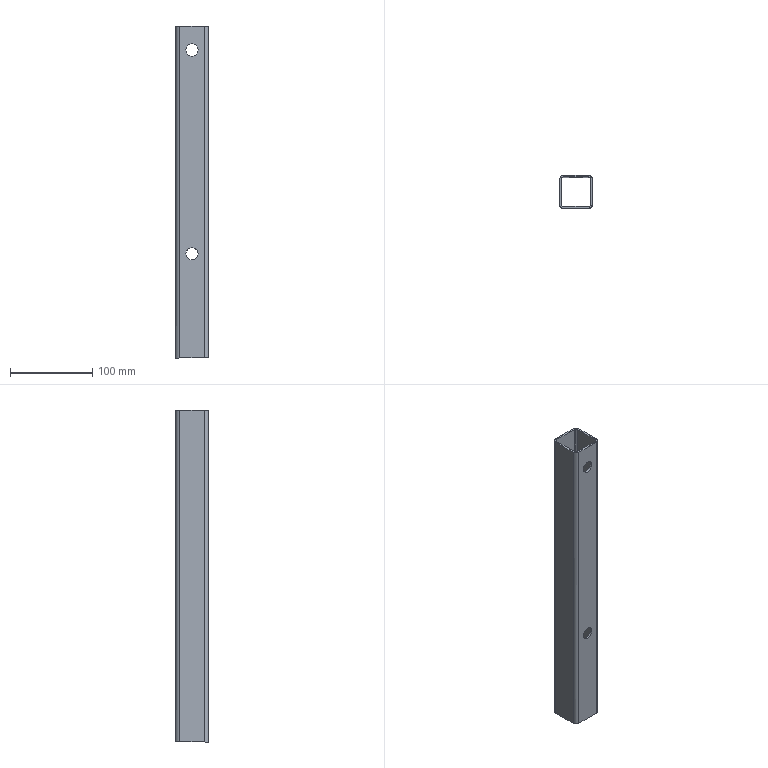Part | NX | features BREP 1 | 1 solid | 30 faces | box 40 x 40 x 404.579 mm | volume 116022 mm3 | cylinder 20 | plane 10 | commonest cylinder face diameters 6 x8 15 x8 10 x4
STEP:
#1=CARTESIAN_POINT('',(2077.08,-390.,484.409));
#2=VERTEX_POINT('',#1);
#3=CARTESIAN_POINT('',(2077.08,-392.,484.409));
#4=VERTEX_POINT('',#3);
#5=CARTESIAN_POINT('',(2077.08,-407.5,484.409));
#6=DIRECTION('',(0.,-1.,0.));
#7=VECTOR('',#6,1000.);
#8=LINE('',#5,#7);
#9=EDGE_CURVE('',#2,#4,#8,.T.);
#10=ORIENTED_EDGE('',*,*,#9,.F.);
#11=CARTESIAN_POINT('',(2092.08,-390.,484.409));
#12=VERTEX_POINT('',#11);
#13=CARTESIAN_POINT('',(2084.58,-390.,484.409));
#14=DIRECTION('',(0.,-1.,0.));
#15=DIRECTION('',(1.,0.,0.));
#16=AXIS2_PLACEMENT_3D('',#13,#14,#15);
#17=CIRCLE('',#16,7.5);
#18=EDGE_CURVE('',#12,#2,#17,.T.);
#19=ORIENTED_EDGE('',*,*,#18,.F.);
#20=CARTESIAN_POINT('',(2092.08,-392.,484.409));
#21=VERTEX_POINT('',#20);
#22=CARTESIAN_POINT('',(2092.08,-407.5,484.409));
#23=DIRECTION('',(0.,-1.,0.));
#24=VECTOR('',#23,1000.);
#25=LINE('',#22,#24);
#26=EDGE_CURVE('',#12,#21,#25,.T.);
#27=ORIENTED_EDGE('',*,*,#26,.T.);
#28=CARTESIAN_POINT('',(2084.58,-392.,484.409));
#29=DIRECTION('',(0.,-1.,0.));
#30=DIRECTION('',(1.,0.,0.));
#31=AXIS2_PLACEMENT_3D('',#28,#29,#30);
#32=CIRCLE('',#31,7.5);
#33=EDGE_CURVE('',#21,#4,#32,.T.);
#34=ORIENTED_EDGE('',*,*,#33,.T.);
#35=EDGE_LOOP('',(#10,#19,#27,#34));
#36=FACE_BOUND('',#35,.T.);
#37=CARTESIAN_POINT('',(2084.58,-407.5,484.409));
#38=DIRECTION('',(0.,-1.,0.));
#39=DIRECTION('',(1.,0.,0.));
#40=AXIS2_PLACEMENT_3D('',#37,#38,#39);
#41=CYLINDRICAL_SURFACE('',#40,7.5);
#42=ADVANCED_FACE('',(#36),#41,.F.);
#43=ORIENTED_EDGE('',*,*,#26,.F.);
#44=CARTESIAN_POINT('',(2084.58,-390.,484.409));
#45=DIRECTION('',(0.,-1.,0.));
#46=DIRECTION('',(1.,0.,0.));
#47=AXIS2_PLACEMENT_3D('',#44,#45,#46);
#48=CIRCLE('',#47,7.5);
#49=EDGE_CURVE('',#2,#12,#48,.T.);
#50=ORIENTED_EDGE('',*,*,#49,.F.);
#51=ORIENTED_EDGE('',*,*,#9,.T.);
#52=CARTESIAN_POINT('',(2084.58,-392.,484.409));
#53=DIRECTION('',(0.,-1.,0.));
#54=DIRECTION('',(1.,0.,0.));
#55=AXIS2_PLACEMENT_3D('',#52,#53,#54);
#56=CIRCLE('',#55,7.5);
#57=EDGE_CURVE('',#4,#21,#56,.T.);
#58=ORIENTED_EDGE('',*,*,#57,.T.);
#59=EDGE_LOOP('',(#43,#50,#51,#58));
#60=FACE_BOUND('',#59,.T.);
#61=CARTESIAN_POINT('',(2084.58,-407.5,484.409));
#62=DIRECTION('',(0.,-1.,0.));
#63=DIRECTION('',(-1.,0.,0.));
#64=AXIS2_PLACEMENT_3D('',#61,#62,#63);
#65=CYLINDRICAL_SURFACE('',#64,7.5);
#66=ADVANCED_FACE('',(#60),#65,.F.);
#67=CARTESIAN_POINT('',(2092.08,-390.,235.999));
#68=VERTEX_POINT('',#67);
#69=CARTESIAN_POINT('',(2092.08,-392.,235.999));
#70=VERTEX_POINT('',#69);
#71=CARTESIAN_POINT('',(2092.08,-407.5,235.999));
#72=DIRECTION('',(0.,1.,0.));
#73=VECTOR('',#72,1000.);
#74=LINE('',#71,#73);
#75=EDGE_CURVE('',#68,#70,#74,.F.);
#76=ORIENTED_EDGE('',*,*,#75,.F.);
#77=CARTESIAN_POINT('',(2077.08,-390.,235.999));
#78=VERTEX_POINT('',#77);
#79=CARTESIAN_POINT('',(2092.08,-390.,235.999));
#80=CARTESIAN_POINT('',(2092.08,-390.,235.195));
#81=CARTESIAN_POINT('',(2091.972,-390.,234.39));
#82=CARTESIAN_POINT('',(2091.756,-390.,233.604));
#83=CARTESIAN_POINT('',(2091.118,-390.,232.11));
#84=CARTESIAN_POINT('',(2090.109,-390.,230.837));
#85=CARTESIAN_POINT('',(2089.522,-390.,230.272));
#86=CARTESIAN_POINT('',(2088.21,-390.,229.314));
#87=CARTESIAN_POINT('',(2086.692,-390.,228.735));
#88=CARTESIAN_POINT('',(2085.899,-390.,228.55));
#89=CARTESIAN_POINT('',(2084.282,-390.,228.397));
#90=CARTESIAN_POINT('',(2082.681,-390.,228.676));
#91=CARTESIAN_POINT('',(2081.905,-390.,228.923));
#92=CARTESIAN_POINT('',(2080.437,-390.,229.618));
#93=CARTESIAN_POINT('',(2079.204,-390.,230.676));
#94=CARTESIAN_POINT('',(2078.663,-390.,231.285));
#95=CARTESIAN_POINT('',(2077.823,-390.,232.535));
#96=CARTESIAN_POINT('',(2077.316,-390.,233.949));
#97=CARTESIAN_POINT('',(2077.158,-390.,234.625));
#98=CARTESIAN_POINT('',(2077.08,-390.,235.312));
#99=CARTESIAN_POINT('',(2077.08,-390.,235.999));
#100=B_SPLINE_CURVE_WITH_KNOTS('',5,(#79,#80,#81,#82,#83,#84,#85,#86,#87,#88,#89,#90,#91,#92,#93,#94,#95,#96,#97,#98,#99),.UNSPECIFIED.,.F.,.F.,(6,3,3,3,3,3,6),(0.,5.692,11.384,17.076,22.768,28.46,33.321),.UNSPECIFIED.);
#101=EDGE_CURVE('',#68,#78,#100,.T.);
#102=ORIENTED_EDGE('',*,*,#101,.T.);
#103=CARTESIAN_POINT('',(2077.08,-392.,235.999));
#104=VERTEX_POINT('',#103);
#105=CARTESIAN_POINT('',(2077.08,-407.5,235.999));
#106=DIRECTION('',(0.,1.,0.));
#107=VECTOR('',#106,1000.);
#108=LINE('',#105,#107);
#109=EDGE_CURVE('',#78,#104,#108,.F.);
#110=ORIENTED_EDGE('',*,*,#109,.T.);
#111=CARTESIAN_POINT('',(2092.08,-392.,235.999));
#112=CARTESIAN_POINT('',(2092.08,-392.,235.195));
#113=CARTESIAN_POINT('',(2091.972,-392.,234.39));
#114=CARTESIAN_POINT('',(2091.756,-392.,233.604));
#115=CARTESIAN_POINT('',(2091.118,-392.,232.11));
#116=CARTESIAN_POINT('',(2090.109,-392.,230.837));
#117=CARTESIAN_POINT('',(2089.522,-392.,230.272));
#118=CARTESIAN_POINT('',(2088.21,-392.,229.314));
#119=CARTESIAN_POINT('',(2086.692,-392.,228.735));
#120=CARTESIAN_POINT('',(2085.899,-392.,228.55));
#121=CARTESIAN_POINT('',(2084.282,-392.,228.397));
#122=CARTESIAN_POINT('',(2082.681,-392.,228.676));
#123=CARTESIAN_POINT('',(2081.905,-392.,228.923));
#124=CARTESIAN_POINT('',(2080.437,-392.,229.618));
#125=CARTESIAN_POINT('',(2079.204,-392.,230.676));
#126=CARTESIAN_POINT('',(2078.663,-392.,231.285));
#127=CARTESIAN_POINT('',(2077.823,-392.,232.535));
#128=CARTESIAN_POINT('',(2077.316,-392.,233.949));
#129=CARTESIAN_POINT('',(2077.158,-392.,234.625));
#130=CARTESIAN_POINT('',(2077.08,-392.,235.312));
#131=CARTESIAN_POINT('',(2077.08,-392.,235.999));
#132=B_SPLINE_CURVE_WITH_KNOTS('',5,(#111,#112,#113,#114,#115,#116,#117,#118,#119,#120,#121,#122,#123,#124,#125,#126,#127,#128,#129,#130,#131),.UNSPECIFIED.,.F.,.F.,(6,3,3,3,3,3,6),(0.,5.692,11.384,17.076,22.768,28.46,33.321),.UNSPECIFIED.);
#133=EDGE_CURVE('',#70,#104,#132,.T.);
#134=ORIENTED_EDGE('',*,*,#133,.F.);
#135=EDGE_LOOP('',(#76,#102,#110,#134));
#136=FACE_BOUND('',#135,.T.);
#137=CARTESIAN_POINT('',(2084.58,-407.5,235.999));
#138=DIRECTION('',(0.,1.,0.));
#139=DIRECTION('',(1.,0.,0.));
#140=AXIS2_PLACEMENT_3D('',#137,#138,#139);
#141=CYLINDRICAL_SURFACE('',#140,7.5);
#142=ADVANCED_FACE('',(#136),#141,.F.);
#143=ORIENTED_EDGE('',*,*,#109,.F.);
#144=CARTESIAN_POINT('',(2077.08,-390.,235.999));
#145=CARTESIAN_POINT('',(2077.08,-390.,236.804));
#146=CARTESIAN_POINT('',(2077.188,-390.,237.609));
#147=CARTESIAN_POINT('',(2077.404,-390.,238.395));
#148=CARTESIAN_POINT('',(2078.041,-390.,239.889));
#149=CARTESIAN_POINT('',(2079.05,-390.,241.162));
#150=CARTESIAN_POINT('',(2079.637,-390.,241.727));
#151=CARTESIAN_POINT('',(2080.949,-390.,242.685));
#152=CARTESIAN_POINT('',(2082.467,-390.,243.264));
#153=CARTESIAN_POINT('',(2083.26,-390.,243.449));
#154=CARTESIAN_POINT('',(2084.878,-390.,243.602));
#155=CARTESIAN_POINT('',(2086.478,-390.,243.323));
#156=CARTESIAN_POINT('',(2087.254,-390.,243.076));
#157=CARTESIAN_POINT('',(2088.722,-390.,242.381));
#158=CARTESIAN_POINT('',(2089.955,-390.,241.323));
#159=CARTESIAN_POINT('',(2090.496,-390.,240.714));
#160=CARTESIAN_POINT('',(2091.336,-390.,239.464));
#161=CARTESIAN_POINT('',(2091.843,-390.,238.05));
#162=CARTESIAN_POINT('',(2092.001,-390.,237.374));
#163=CARTESIAN_POINT('',(2092.08,-390.,236.687));
#164=CARTESIAN_POINT('',(2092.08,-390.,235.999));
#165=B_SPLINE_CURVE_WITH_KNOTS('',5,(#144,#145,#146,#147,#148,#149,#150,#151,#152,#153,#154,#155,#156,#157,#158,#159,#160,#161,#162,#163,#164),.UNSPECIFIED.,.F.,.F.,(6,3,3,3,3,3,6),(0.,5.692,11.384,17.076,22.768,28.46,33.321),.UNSPECIFIED.);
#166=EDGE_CURVE('',#78,#68,#165,.T.);
#167=ORIENTED_EDGE('',*,*,#166,.T.);
#168=ORIENTED_EDGE('',*,*,#75,.T.);
#169=CARTESIAN_POINT('',(2077.08,-392.,235.999));
#170=CARTESIAN_POINT('',(2077.08,-392.,236.804));
#171=CARTESIAN_POINT('',(2077.188,-392.,237.609));
#172=CARTESIAN_POINT('',(2077.404,-392.,238.395));
#173=CARTESIAN_POINT('',(2078.041,-392.,239.889));
#174=CARTESIAN_POINT('',(2079.05,-392.,241.162));
#175=CARTESIAN_POINT('',(2079.637,-392.,241.727));
#176=CARTESIAN_POINT('',(2080.949,-392.,242.685));
#177=CARTESIAN_POINT('',(2082.467,-392.,243.264));
#178=CARTESIAN_POINT('',(2083.26,-392.,243.449));
#179=CARTESIAN_POINT('',(2084.878,-392.,243.602));
#180=CARTESIAN_POINT('',(2086.478,-392.,243.323));
#181=CARTESIAN_POINT('',(2087.254,-392.,243.076));
#182=CARTESIAN_POINT('',(2088.722,-392.,242.381));
#183=CARTESIAN_POINT('',(2089.955,-392.,241.323));
#184=CARTESIAN_POINT('',(2090.496,-392.,240.714));
#185=CARTESIAN_POINT('',(2091.336,-392.,239.464));
#186=CARTESIAN_POINT('',(2091.843,-392.,238.05));
#187=CARTESIAN_POINT('',(2092.001,-392.,237.374));
#188=CARTESIAN_POINT('',(2092.08,-392.,236.687));
#189=CARTESIAN_POINT('',(2092.08,-392.,235.999));
#190=B_SPLINE_CURVE_WITH_KNOTS('',5,(#169,#170,#171,#172,#173,#174,#175,#176,#177,#178,#179,#180,#181,#182,#183,#184,#185,#186,#187,#188,#189),.UNSPECIFIED.,.F.,.F.,(6,3,3,3,3,3,6),(0.,5.692,11.384,17.076,22.768,28.46,33.321),.UNSPECIFIED.);
#191=EDGE_CURVE('',#104,#70,#190,.T.);
#192=ORIENTED_EDGE('',*,*,#191,.F.);
#193=EDGE_LOOP('',(#143,#167,#168,#192));
#194=FACE_BOUND('',#193,.T.);
#195=CARTESIAN_POINT('',(2084.58,-407.5,235.999));
#196=DIRECTION('',(0.,1.,0.));
#197=DIRECTION('',(-1.,0.,0.));
#198=AXIS2_PLACEMENT_3D('',#195,#196,#197);
#199=CYLINDRICAL_SURFACE('',#198,7.5);
#200=ADVANCED_FACE('',(#194),#199,.F.);
#201=CARTESIAN_POINT('',(2102.58,-395.,109.));
#202=VERTEX_POINT('',#201);
#203=CARTESIAN_POINT('',(2101.701,-392.879,109.));
#204=VERTEX_POINT('',#203);
#205=CARTESIAN_POINT('',(2099.58,-395.,109.));
#206=DIRECTION('',(0.,0.,1.));
#207=DIRECTION('',(1.,0.,0.));
#208=AXIS2_PLACEMENT_3D('',#205,#206,#207);
#209=CIRCLE('',#208,3.);
#210=EDGE_CURVE('',#202,#204,#209,.T.);
#211=ORIENTED_EDGE('',*,*,#210,.F.);
#212=CARTESIAN_POINT('',(2102.58,-395.,513.579));
#213=VERTEX_POINT('',#212);
#214=CARTESIAN_POINT('',(2102.58,-395.,311.29));
#215=DIRECTION('',(0.,0.,-1.));
#216=VECTOR('',#215,1000.);
#217=LINE('',#214,#216);
#218=EDGE_CURVE('',#213,#202,#217,.T.);
#219=ORIENTED_EDGE('',*,*,#218,.F.);
#220=CARTESIAN_POINT('',(2101.701,-392.879,513.579));
#221=VERTEX_POINT('',#220);
#222=CARTESIAN_POINT('',(2101.701,-392.879,513.579));
#223=CARTESIAN_POINT('',(2101.848,-393.025,513.579));
#224=CARTESIAN_POINT('',(2101.982,-393.185,513.579));
#225=CARTESIAN_POINT('',(2102.102,-393.356,513.579));
#226=CARTESIAN_POINT('',(2102.339,-393.765,513.579));
#227=CARTESIAN_POINT('',(2102.493,-394.213,513.579));
#228=CARTESIAN_POINT('',(2102.551,-394.473,513.579));
#229=CARTESIAN_POINT('',(2102.58,-394.736,513.579));
#230=CARTESIAN_POINT('',(2102.58,-395.,513.579));
#231=B_SPLINE_CURVE_WITH_KNOTS('',5,(#222,#223,#224,#225,#226,#227,#228,#229,#230),.UNSPECIFIED.,.F.,.F.,(6,3,6),(3.332,4.8,6.664),.UNSPECIFIED.);
#232=EDGE_CURVE('',#221,#213,#231,.T.);
#233=ORIENTED_EDGE('',*,*,#232,.F.);
#234=CARTESIAN_POINT('',(2101.701,-392.879,360.204));
#235=DIRECTION('',(0.,0.,-1.));
#236=VECTOR('',#235,1000.);
#237=LINE('',#234,#236);
#238=EDGE_CURVE('',#221,#204,#237,.T.);
#239=ORIENTED_EDGE('',*,*,#238,.T.);
#240=EDGE_LOOP('',(#211,#219,#233,#239));
#241=FACE_BOUND('',#240,.T.);
#242=CARTESIAN_POINT('',(2099.58,-395.,360.204));
#243=DIRECTION('',(0.,0.,-1.));
#244=DIRECTION('',(0.7071,0.7071,0.));
#245=AXIS2_PLACEMENT_3D('',#242,#243,#244);
#246=CYLINDRICAL_SURFACE('',#245,3.);
#247=ADVANCED_FACE('',(#241),#246,.F.);
#248=CARTESIAN_POINT('',(2099.58,-392.,513.579));
#249=VERTEX_POINT('',#248);
#250=CARTESIAN_POINT('',(2099.58,-392.,513.579));
#251=CARTESIAN_POINT('',(2099.919,-392.,513.579));
#252=CARTESIAN_POINT('',(2100.258,-392.048,513.579));
#253=CARTESIAN_POINT('',(2100.589,-392.144,513.579));
#254=CARTESIAN_POINT('',(2101.022,-392.34,513.579));
#255=CARTESIAN_POINT('',(2101.406,-392.615,513.579));
#256=CARTESIAN_POINT('',(2101.509,-392.697,513.579));
#257=CARTESIAN_POINT('',(2101.608,-392.785,513.579));
#258=CARTESIAN_POINT('',(2101.701,-392.879,513.579));
#259=B_SPLINE_CURVE_WITH_KNOTS('',5,(#250,#251,#252,#253,#254,#255,#256,#257,#258),.UNSPECIFIED.,.F.,.F.,(6,3,6),(0.,2.4,3.332),.UNSPECIFIED.);
#260=EDGE_CURVE('',#249,#221,#259,.T.);
#261=ORIENTED_EDGE('',*,*,#260,.F.);
#262=CARTESIAN_POINT('',(2099.58,-392.,109.));
#263=VERTEX_POINT('',#262);
#264=CARTESIAN_POINT('',(2099.58,-392.,311.29));
#265=DIRECTION('',(0.,0.,-1.));
#266=VECTOR('',#265,1000.);
#267=LINE('',#264,#266);
#268=EDGE_CURVE('',#249,#263,#267,.T.);
#269=ORIENTED_EDGE('',*,*,#268,.T.);
#270=CARTESIAN_POINT('',(2099.58,-395.,109.));
#271=DIRECTION('',(0.,0.,1.));
#272=DIRECTION('',(1.,0.,0.));
#273=AXIS2_PLACEMENT_3D('',#270,#271,#272);
#274=CIRCLE('',#273,3.);
#275=EDGE_CURVE('',#204,#263,#274,.T.);
#276=ORIENTED_EDGE('',*,*,#275,.F.);
#277=ORIENTED_EDGE('',*,*,#238,.F.);
#278=EDGE_LOOP('',(#261,#269,#276,#277));
#279=FACE_BOUND('',#278,.T.);
#280=CARTESIAN_POINT('',(2099.58,-395.,360.204));
#281=DIRECTION('',(0.,0.,-1.));
#282=DIRECTION('',(-0.7071,-0.7071,0.));
#283=AXIS2_PLACEMENT_3D('',#280,#281,#282);
#284=CYLINDRICAL_SURFACE('',#283,3.);
#285=ADVANCED_FACE('',(#279),#284,.F.);
#286=ORIENTED_EDGE('',*,*,#33,.F.);
#287=ORIENTED_EDGE('',*,*,#57,.F.);
#288=EDGE_LOOP('',(#286,#287));
#289=FACE_BOUND('',#288,.T.);
#290=ORIENTED_EDGE('',*,*,#133,.T.);
#291=ORIENTED_EDGE('',*,*,#191,.T.);
#292=EDGE_LOOP('',(#290,#291));
#293=FACE_BOUND('',#292,.T.);
#294=CARTESIAN_POINT('',(2069.58,-392.,513.579));
#295=VERTEX_POINT('',#294);
#296=CARTESIAN_POINT('',(2069.58,-392.,109.));
#297=VERTEX_POINT('',#296);
#298=CARTESIAN_POINT('',(2069.58,-392.,360.204));
#299=DIRECTION('',(0.,0.,-1.));
#300=VECTOR('',#299,1000.);
#301=LINE('',#298,#300);
#302=EDGE_CURVE('',#295,#297,#301,.T.);
#303=ORIENTED_EDGE('',*,*,#302,.T.);
#304=CARTESIAN_POINT('',(2084.58,-392.,109.));
#305=DIRECTION('',(-1.,0.,0.));
#306=VECTOR('',#305,1000.);
#307=LINE('',#304,#306);
#308=EDGE_CURVE('',#263,#297,#307,.T.);
#309=ORIENTED_EDGE('',*,*,#308,.F.);
#310=ORIENTED_EDGE('',*,*,#268,.F.);
#311=CARTESIAN_POINT('',(2084.58,-392.,513.579));
#312=DIRECTION('',(-1.,0.,0.));
#313=VECTOR('',#312,1000.);
#314=LINE('',#311,#313);
#315=EDGE_CURVE('',#249,#295,#314,.T.);
#316=ORIENTED_EDGE('',*,*,#315,.T.);
#317=EDGE_LOOP('',(#303,#309,#310,#316));
#318=FACE_BOUND('',#317,.T.);
#319=CARTESIAN_POINT('',(2104.58,-392.,534.409));
#320=DIRECTION('',(0.,-1.,0.));
#321=DIRECTION('',(-1.,0.,0.));
#322=AXIS2_PLACEMENT_3D('',#319,#320,#321);
#323=PLANE('',#322);
#324=ADVANCED_FACE('',(#289,#293,#318),#323,.T.);
#325=CARTESIAN_POINT('',(2067.458,-392.879,109.));
#326=VERTEX_POINT('',#325);
#327=CARTESIAN_POINT('',(2069.58,-395.,109.));
#328=DIRECTION('',(0.,0.,1.));
#329=DIRECTION('',(1.,0.,0.));
#330=AXIS2_PLACEMENT_3D('',#327,#328,#329);
#331=CIRCLE('',#330,3.);
#332=EDGE_CURVE('',#297,#326,#331,.T.);
#333=ORIENTED_EDGE('',*,*,#332,.F.);
#334=ORIENTED_EDGE('',*,*,#302,.F.);
#335=CARTESIAN_POINT('',(2067.458,-392.879,513.579));
#336=VERTEX_POINT('',#335);
#337=CARTESIAN_POINT('',(2067.458,-392.879,513.579));
#338=CARTESIAN_POINT('',(2067.605,-392.732,513.579));
#339=CARTESIAN_POINT('',(2067.765,-392.598,513.579));
#340=CARTESIAN_POINT('',(2067.935,-392.478,513.579));
#341=CARTESIAN_POINT('',(2068.344,-392.241,513.579));
#342=CARTESIAN_POINT('',(2068.793,-392.087,513.579));
#343=CARTESIAN_POINT('',(2069.052,-392.029,513.579));
#344=CARTESIAN_POINT('',(2069.316,-392.,513.579));
#345=CARTESIAN_POINT('',(2069.58,-392.,513.579));
#346=B_SPLINE_CURVE_WITH_KNOTS('',5,(#337,#338,#339,#340,#341,#342,#343,#344,#345),.UNSPECIFIED.,.F.,.F.,(6,3,6),(3.332,4.8,6.664),.UNSPECIFIED.);
#347=EDGE_CURVE('',#336,#295,#346,.T.);
#348=ORIENTED_EDGE('',*,*,#347,.F.);
#349=CARTESIAN_POINT('',(2067.458,-392.879,360.204));
#350=DIRECTION('',(0.,0.,-1.));
#351=VECTOR('',#350,1000.);
#352=LINE('',#349,#351);
#353=EDGE_CURVE('',#336,#326,#352,.T.);
#354=ORIENTED_EDGE('',*,*,#353,.T.);
#355=EDGE_LOOP('',(#333,#334,#348,#354));
#356=FACE_BOUND('',#355,.T.);
#357=CARTESIAN_POINT('',(2069.58,-395.,360.204));
#358=DIRECTION('',(0.,0.,-1.));
#359=DIRECTION('',(-0.7071,0.7071,0.));
#360=AXIS2_PLACEMENT_3D('',#357,#358,#359);
#361=CYLINDRICAL_SURFACE('',#360,3.);
#362=ADVANCED_FACE('',(#356),#361,.F.);
#363=CARTESIAN_POINT('',(2066.58,-395.,513.579));
#364=VERTEX_POINT('',#363);
#365=CARTESIAN_POINT('',(2066.58,-395.,513.579));
#366=CARTESIAN_POINT('',(2066.58,-394.661,513.579));
#367=CARTESIAN_POINT('',(2066.628,-394.321,513.579));
#368=CARTESIAN_POINT('',(2066.724,-393.991,513.579));
#369=CARTESIAN_POINT('',(2066.92,-393.557,513.579));
#370=CARTESIAN_POINT('',(2067.194,-393.173,513.579));
#371=CARTESIAN_POINT('',(2067.277,-393.07,513.579));
#372=CARTESIAN_POINT('',(2067.365,-392.972,513.579));
#373=CARTESIAN_POINT('',(2067.458,-392.879,513.579));
#374=B_SPLINE_CURVE_WITH_KNOTS('',5,(#365,#366,#367,#368,#369,#370,#371,#372,#373),.UNSPECIFIED.,.F.,.F.,(6,3,6),(0.,2.4,3.332),.UNSPECIFIED.);
#375=EDGE_CURVE('',#364,#336,#374,.T.);
#376=ORIENTED_EDGE('',*,*,#375,.F.);
#377=CARTESIAN_POINT('',(2066.58,-395.,109.));
#378=VERTEX_POINT('',#377);
#379=CARTESIAN_POINT('',(2066.58,-395.,311.29));
#380=DIRECTION('',(0.,0.,-1.));
#381=VECTOR('',#380,1000.);
#382=LINE('',#379,#381);
#383=EDGE_CURVE('',#364,#378,#382,.T.);
#384=ORIENTED_EDGE('',*,*,#383,.T.);
#385=CARTESIAN_POINT('',(2069.58,-395.,109.));
#386=DIRECTION('',(0.,0.,1.));
#387=DIRECTION('',(1.,0.,0.));
#388=AXIS2_PLACEMENT_3D('',#385,#386,#387);
#389=CIRCLE('',#388,3.);
#390=EDGE_CURVE('',#326,#378,#389,.T.);
#391=ORIENTED_EDGE('',*,*,#390,.F.);
#392=ORIENTED_EDGE('',*,*,#353,.F.);
#393=EDGE_LOOP('',(#376,#384,#391,#392));
#394=FACE_BOUND('',#393,.T.);
#395=CARTESIAN_POINT('',(2069.58,-395.,360.204));
#396=DIRECTION('',(0.,0.,-1.));
#397=DIRECTION('',(0.7071,-0.7071,0.));
#398=AXIS2_PLACEMENT_3D('',#395,#396,#397);
#399=CYLINDRICAL_SURFACE('',#398,3.);
#400=ADVANCED_FACE('',(#394),#399,.F.);
#401=CARTESIAN_POINT('',(2066.58,-425.,513.579));
#402=VERTEX_POINT('',#401);
#403=CARTESIAN_POINT('',(2066.58,-410.,513.579));
#404=DIRECTION('',(0.,1.,0.));
#405=VECTOR('',#404,1000.);
#406=LINE('',#403,#405);
#407=EDGE_CURVE('',#402,#364,#406,.T.);
#408=ORIENTED_EDGE('',*,*,#407,.F.);
#409=CARTESIAN_POINT('',(2066.58,-425.,109.));
#410=VERTEX_POINT('',#409);
#411=CARTESIAN_POINT('',(2066.58,-425.,360.204));
#412=DIRECTION('',(0.,0.,-1.));
#413=VECTOR('',#412,1000.);
#414=LINE('',#411,#413);
#415=EDGE_CURVE('',#402,#410,#414,.T.);
#416=ORIENTED_EDGE('',*,*,#415,.T.);
#417=CARTESIAN_POINT('',(2066.58,-410.,109.));
#418=DIRECTION('',(0.,1.,0.));
#419=VECTOR('',#418,1000.);
#420=LINE('',#417,#419);
#421=EDGE_CURVE('',#410,#378,#420,.T.);
#422=ORIENTED_EDGE('',*,*,#421,.T.);
#423=ORIENTED_EDGE('',*,*,#383,.F.);
#424=EDGE_LOOP('',(#408,#416,#422,#423));
#425=FACE_BOUND('',#424,.T.);
#426=CARTESIAN_POINT('',(2066.58,-430.,534.409));
#427=DIRECTION('',(-1.,0.,0.));
#428=DIRECTION('',(0.,1.,0.));
#429=AXIS2_PLACEMENT_3D('',#426,#427,#428);
#430=PLANE('',#429);
#431=ADVANCED_FACE('',(#425),#430,.F.);
#432=CARTESIAN_POINT('',(2067.458,-427.121,109.));
#433=VERTEX_POINT('',#432);
#434=CARTESIAN_POINT('',(2069.58,-425.,109.));
#435=DIRECTION('',(0.,0.,1.));
#436=DIRECTION('',(1.,0.,0.));
#437=AXIS2_PLACEMENT_3D('',#434,#435,#436);
#438=CIRCLE('',#437,3.);
#439=EDGE_CURVE('',#410,#433,#438,.T.);
#440=ORIENTED_EDGE('',*,*,#439,.F.);
#441=ORIENTED_EDGE('',*,*,#415,.F.);
#442=CARTESIAN_POINT('',(2067.458,-427.121,513.579));
#443=VERTEX_POINT('',#442);
#444=CARTESIAN_POINT('',(2067.458,-427.121,513.579));
#445=CARTESIAN_POINT('',(2067.312,-426.975,513.579));
#446=CARTESIAN_POINT('',(2067.177,-426.815,513.579));
#447=CARTESIAN_POINT('',(2067.057,-426.644,513.579));
#448=CARTESIAN_POINT('',(2066.82,-426.235,513.579));
#449=CARTESIAN_POINT('',(2066.667,-425.787,513.579));
#450=CARTESIAN_POINT('',(2066.609,-425.527,513.579));
#451=CARTESIAN_POINT('',(2066.58,-425.264,513.579));
#452=CARTESIAN_POINT('',(2066.58,-425.,513.579));
#453=B_SPLINE_CURVE_WITH_KNOTS('',5,(#444,#445,#446,#447,#448,#449,#450,#451,#452),.UNSPECIFIED.,.F.,.F.,(6,3,6),(3.332,4.8,6.664),.UNSPECIFIED.);
#454=EDGE_CURVE('',#443,#402,#453,.T.);
#455=ORIENTED_EDGE('',*,*,#454,.F.);
#456=CARTESIAN_POINT('',(2067.458,-427.121,360.204));
#457=DIRECTION('',(0.,0.,-1.));
#458=VECTOR('',#457,1000.);
#459=LINE('',#456,#458);
#460=EDGE_CURVE('',#443,#433,#459,.T.);
#461=ORIENTED_EDGE('',*,*,#460,.T.);
#462=EDGE_LOOP('',(#440,#441,#455,#461));
#463=FACE_BOUND('',#462,.T.);
#464=CARTESIAN_POINT('',(2069.58,-425.,360.204));
#465=DIRECTION('',(0.,0.,-1.));
#466=DIRECTION('',(-0.7071,-0.7071,0.));
#467=AXIS2_PLACEMENT_3D('',#464,#465,#466);
#468=CYLINDRICAL_SURFACE('',#467,3.);
#469=ADVANCED_FACE('',(#463),#468,.F.);
#470=CARTESIAN_POINT('',(2102.58,-425.,513.579));
#471=VERTEX_POINT('',#470);
#472=CARTESIAN_POINT('',(2101.701,-427.121,513.579));
#473=VERTEX_POINT('',#472);
#474=CARTESIAN_POINT('',(2102.58,-425.,513.579));
#475=CARTESIAN_POINT('',(2102.58,-425.339,513.579));
#476=CARTESIAN_POINT('',(2102.532,-425.679,513.579));
#477=CARTESIAN_POINT('',(2102.436,-426.009,513.579));
#478=CARTESIAN_POINT('',(2102.239,-426.443,513.579));
#479=CARTESIAN_POINT('',(2101.965,-426.827,513.579));
#480=CARTESIAN_POINT('',(2101.882,-426.93,513.579));
#481=CARTESIAN_POINT('',(2101.794,-427.028,513.579));
#482=CARTESIAN_POINT('',(2101.701,-427.121,513.579));
#483=B_SPLINE_CURVE_WITH_KNOTS('',5,(#474,#475,#476,#477,#478,#479,#480,#481,#482),.UNSPECIFIED.,.F.,.F.,(6,3,6),(0.,2.4,3.332),.UNSPECIFIED.);
#484=EDGE_CURVE('',#471,#473,#483,.T.);
#485=ORIENTED_EDGE('',*,*,#484,.F.);
#486=CARTESIAN_POINT('',(2102.58,-425.,109.));
#487=VERTEX_POINT('',#486);
#488=CARTESIAN_POINT('',(2102.58,-425.,311.29));
#489=DIRECTION('',(0.,0.,-1.));
#490=VECTOR('',#489,1000.);
#491=LINE('',#488,#490);
#492=EDGE_CURVE('',#471,#487,#491,.T.);
#493=ORIENTED_EDGE('',*,*,#492,.T.);
#494=CARTESIAN_POINT('',(2101.701,-427.121,109.));
#495=VERTEX_POINT('',#494);
#496=CARTESIAN_POINT('',(2099.58,-425.,109.));
#497=DIRECTION('',(0.,0.,1.));
#498=DIRECTION('',(1.,0.,0.));
#499=AXIS2_PLACEMENT_3D('',#496,#497,#498);
#500=CIRCLE('',#499,3.);
#501=EDGE_CURVE('',#495,#487,#500,.T.);
#502=ORIENTED_EDGE('',*,*,#501,.F.);
#503=CARTESIAN_POINT('',(2101.701,-427.121,360.204));
#504=DIRECTION('',(0.,0.,-1.));
#505=VECTOR('',#504,1000.);
#506=LINE('',#503,#505);
#507=EDGE_CURVE('',#473,#495,#506,.T.);
#508=ORIENTED_EDGE('',*,*,#507,.F.);
#509=EDGE_LOOP('',(#485,#493,#502,#508));
#510=FACE_BOUND('',#509,.T.);
#511=CARTESIAN_POINT('',(2099.58,-425.,360.204));
#512=DIRECTION('',(0.,0.,-1.));
#513=DIRECTION('',(-0.7071,0.7071,0.));
#514=AXIS2_PLACEMENT_3D('',#511,#512,#513);
#515=CYLINDRICAL_SURFACE('',#514,3.);
#516=ADVANCED_FACE('',(#510),#515,.F.);
#517=CARTESIAN_POINT('',(2102.58,-410.,513.579));
#518=DIRECTION('',(0.,-1.,0.));
#519=VECTOR('',#518,1000.);
#520=LINE('',#517,#519);
#521=EDGE_CURVE('',#213,#471,#520,.T.);
#522=ORIENTED_EDGE('',*,*,#521,.F.);
#523=ORIENTED_EDGE('',*,*,#218,.T.);
#524=CARTESIAN_POINT('',(2102.58,-410.,109.));
#525=DIRECTION('',(0.,-1.,0.));
#526=VECTOR('',#525,1000.);
#527=LINE('',#524,#526);
#528=EDGE_CURVE('',#202,#487,#527,.T.);
#529=ORIENTED_EDGE('',*,*,#528,.T.);
#530=ORIENTED_EDGE('',*,*,#492,.F.);
#531=EDGE_LOOP('',(#522,#523,#529,#530));
#532=FACE_BOUND('',#531,.T.);
#533=CARTESIAN_POINT('',(2102.58,-390.,534.409));
#534=DIRECTION('',(1.,0.,0.));
#535=DIRECTION('',(0.,-1.,0.));
#536=AXIS2_PLACEMENT_3D('',#533,#534,#535);
#537=PLANE('',#536);
#538=ADVANCED_FACE('',(#532),#537,.F.);
#539=CARTESIAN_POINT('',(2064.58,-395.,513.579));
#540=VERTEX_POINT('',#539);
#541=CARTESIAN_POINT('',(2064.58,-395.,109.));
#542=VERTEX_POINT('',#541);
#543=CARTESIAN_POINT('',(2064.58,-395.,360.204));
#544=DIRECTION('',(0.,0.,-1.));
#545=VECTOR('',#544,1000.);
#546=LINE('',#543,#545);
#547=EDGE_CURVE('',#540,#542,#546,.T.);
#548=ORIENTED_EDGE('',*,*,#547,.T.);
#549=CARTESIAN_POINT('',(2064.58,-425.,109.));
#550=VERTEX_POINT('',#549);
#551=CARTESIAN_POINT('',(2064.58,-410.,109.));
#552=DIRECTION('',(0.,1.,0.));
#553=VECTOR('',#552,1000.);
#554=LINE('',#551,#553);
#555=EDGE_CURVE('',#550,#542,#554,.T.);
#556=ORIENTED_EDGE('',*,*,#555,.F.);
#557=CARTESIAN_POINT('',(2064.58,-425.,513.579));
#558=VERTEX_POINT('',#557);
#559=CARTESIAN_POINT('',(2064.58,-425.,360.204));
#560=DIRECTION('',(0.,0.,-1.));
#561=VECTOR('',#560,1000.);
#562=LINE('',#559,#561);
#563=EDGE_CURVE('',#558,#550,#562,.T.);
#564=ORIENTED_EDGE('',*,*,#563,.F.);
#565=CARTESIAN_POINT('',(2064.58,-410.,513.579));
#566=DIRECTION('',(0.,1.,0.));
#567=VECTOR('',#566,1000.);
#568=LINE('',#565,#567);
#569=EDGE_CURVE('',#558,#540,#568,.T.);
#570=ORIENTED_EDGE('',*,*,#569,.T.);
#571=EDGE_LOOP('',(#548,#556,#564,#570));
#572=FACE_BOUND('',#571,.T.);
#573=CARTESIAN_POINT('',(2064.58,-430.,534.409));
#574=DIRECTION('',(-1.,0.,0.));
#575=DIRECTION('',(0.,1.,0.));
#576=AXIS2_PLACEMENT_3D('',#573,#574,#575);
#577=PLANE('',#576);
#578=ADVANCED_FACE('',(#572),#577,.T.);
#579=CARTESIAN_POINT('',(2069.58,-390.,513.579));
#580=VERTEX_POINT('',#579);
#581=CARTESIAN_POINT('',(2069.58,-390.,109.));
#582=VERTEX_POINT('',#581);
#583=CARTESIAN_POINT('',(2069.58,-390.,311.29));
#584=DIRECTION('',(0.,0.,-1.));
#585=VECTOR('',#584,1000.);
#586=LINE('',#583,#585);
#587=EDGE_CURVE('',#580,#582,#586,.T.);
#588=ORIENTED_EDGE('',*,*,#587,.T.);
#589=CARTESIAN_POINT('',(2069.58,-395.,109.));
#590=DIRECTION('',(0.,0.,1.));
#591=DIRECTION('',(1.,0.,0.));
#592=AXIS2_PLACEMENT_3D('',#589,#590,#591);
#593=CIRCLE('',#592,5.);
#594=EDGE_CURVE('',#582,#542,#593,.T.);
#595=ORIENTED_EDGE('',*,*,#594,.T.);
#596=ORIENTED_EDGE('',*,*,#547,.F.);
#597=CARTESIAN_POINT('',(2064.58,-395.,513.579));
#598=CARTESIAN_POINT('',(2064.58,-394.452,513.579));
#599=CARTESIAN_POINT('',(2064.655,-393.905,513.579));
#600=CARTESIAN_POINT('',(2064.805,-393.371,513.579));
#601=CARTESIAN_POINT('',(2065.247,-392.357,513.579));
#602=CARTESIAN_POINT('',(2065.946,-391.5,513.579));
#603=CARTESIAN_POINT('',(2066.352,-391.122,513.579));
#604=CARTESIAN_POINT('',(2067.197,-390.53,513.579));
#605=CARTESIAN_POINT('',(2068.162,-390.169,513.579));
#606=CARTESIAN_POINT('',(2068.629,-390.056,513.579));
#607=CARTESIAN_POINT('',(2069.104,-390.,513.579));
#608=CARTESIAN_POINT('',(2069.58,-390.,513.579));
#609=B_SPLINE_CURVE_WITH_KNOTS('',5,(#597,#598,#599,#600,#601,#602,#603,#604,#605,#606,#607,#608),.UNSPECIFIED.,.F.,.F.,(6,3,3,6),(0.,3.873,7.746,11.107),.UNSPECIFIED.);
#610=EDGE_CURVE('',#540,#580,#609,.T.);
#611=ORIENTED_EDGE('',*,*,#610,.T.);
#612=EDGE_LOOP('',(#588,#595,#596,#611));
#613=FACE_BOUND('',#612,.T.);
#614=CARTESIAN_POINT('',(2069.58,-395.,360.204));
#615=DIRECTION('',(0.,0.,-1.));
#616=DIRECTION('',(-1.,0.,0.));
#617=AXIS2_PLACEMENT_3D('',#614,#615,#616);
#618=CYLINDRICAL_SURFACE('',#617,5.);
#619=ADVANCED_FACE('',(#613),#618,.T.);
#620=ORIENTED_EDGE('',*,*,#49,.T.);
#621=ORIENTED_EDGE('',*,*,#18,.T.);
#622=EDGE_LOOP('',(#620,#621));
#623=FACE_BOUND('',#622,.T.);
#624=ORIENTED_EDGE('',*,*,#166,.F.);
#625=ORIENTED_EDGE('',*,*,#101,.F.);
#626=EDGE_LOOP('',(#624,#625));
#627=FACE_BOUND('',#626,.T.);
#628=CARTESIAN_POINT('',(2099.58,-390.,513.579));
#629=VERTEX_POINT('',#628);
#630=CARTESIAN_POINT('',(2084.58,-390.,513.579));
#631=DIRECTION('',(-1.,0.,0.));
#632=VECTOR('',#631,1000.);
#633=LINE('',#630,#632);
#634=EDGE_CURVE('',#629,#580,#633,.T.);
#635=ORIENTED_EDGE('',*,*,#634,.F.);
#636=CARTESIAN_POINT('',(2099.58,-390.,109.));
#637=VERTEX_POINT('',#636);
#638=CARTESIAN_POINT('',(2099.58,-390.,360.204));
#639=DIRECTION('',(0.,0.,-1.));
#640=VECTOR('',#639,1000.);
#641=LINE('',#638,#640);
#642=EDGE_CURVE('',#629,#637,#641,.T.);
#643=ORIENTED_EDGE('',*,*,#642,.T.);
#644=CARTESIAN_POINT('',(2084.58,-390.,109.));
#645=DIRECTION('',(-1.,0.,0.));
#646=VECTOR('',#645,1000.);
#647=LINE('',#644,#646);
#648=EDGE_CURVE('',#637,#582,#647,.T.);
#649=ORIENTED_EDGE('',*,*,#648,.T.);
#650=ORIENTED_EDGE('',*,*,#587,.F.);
#651=EDGE_LOOP('',(#635,#643,#649,#650));
#652=FACE_BOUND('',#651,.T.);
#653=CARTESIAN_POINT('',(2104.58,-390.,534.409));
#654=DIRECTION('',(0.,-1.,0.));
#655=DIRECTION('',(-1.,0.,0.));
#656=AXIS2_PLACEMENT_3D('',#653,#654,#655);
#657=PLANE('',#656);
#658=ADVANCED_FACE('',(#623,#627,#652),#657,.F.);
#659=CARTESIAN_POINT('',(2104.58,-395.,513.579));
#660=VERTEX_POINT('',#659);
#661=CARTESIAN_POINT('',(2104.58,-395.,109.));
#662=VERTEX_POINT('',#661);
#663=CARTESIAN_POINT('',(2104.58,-395.,311.29));
#664=DIRECTION('',(0.,0.,-1.));
#665=VECTOR('',#664,1000.);
#666=LINE('',#663,#665);
#667=EDGE_CURVE('',#660,#662,#666,.T.);
#668=ORIENTED_EDGE('',*,*,#667,.T.);
#669=CARTESIAN_POINT('',(2099.58,-395.,109.));
#670=DIRECTION('',(0.,0.,1.));
#671=DIRECTION('',(1.,0.,0.));
#672=AXIS2_PLACEMENT_3D('',#669,#670,#671);
#673=CIRCLE('',#672,5.);
#674=EDGE_CURVE('',#662,#637,#673,.T.);
#675=ORIENTED_EDGE('',*,*,#674,.T.);
#676=ORIENTED_EDGE('',*,*,#642,.F.);
#677=CARTESIAN_POINT('',(2099.58,-390.,513.579));
#678=CARTESIAN_POINT('',(2100.127,-390.,513.579));
#679=CARTESIAN_POINT('',(2100.675,-390.075,513.579));
#680=CARTESIAN_POINT('',(2101.209,-390.225,513.579));
#681=CARTESIAN_POINT('',(2102.222,-390.667,513.579));
#682=CARTESIAN_POINT('',(2103.079,-391.366,513.579));
#683=CARTESIAN_POINT('',(2103.457,-391.772,513.579));
#684=CARTESIAN_POINT('',(2104.05,-392.618,513.579));
#685=CARTESIAN_POINT('',(2104.41,-393.583,513.579));
#686=CARTESIAN_POINT('',(2104.523,-394.049,513.579));
#687=CARTESIAN_POINT('',(2104.58,-394.525,513.579));
#688=CARTESIAN_POINT('',(2104.58,-395.,513.579));
#689=B_SPLINE_CURVE_WITH_KNOTS('',5,(#677,#678,#679,#680,#681,#682,#683,#684,#685,#686,#687,#688),.UNSPECIFIED.,.F.,.F.,(6,3,3,6),(0.,3.873,7.746,11.107),.UNSPECIFIED.);
#690=EDGE_CURVE('',#629,#660,#689,.T.);
#691=ORIENTED_EDGE('',*,*,#690,.T.);
#692=EDGE_LOOP('',(#668,#675,#676,#691));
#693=FACE_BOUND('',#692,.T.);
#694=CARTESIAN_POINT('',(2099.58,-395.,360.204));
#695=DIRECTION('',(0.,0.,-1.));
#696=DIRECTION('',(0.,1.,0.));
#697=AXIS2_PLACEMENT_3D('',#694,#695,#696);
#698=CYLINDRICAL_SURFACE('',#697,5.);
#699=ADVANCED_FACE('',(#693),#698,.T.);
#700=CARTESIAN_POINT('',(2104.58,-425.,513.579));
#701=VERTEX_POINT('',#700);
#702=CARTESIAN_POINT('',(2104.58,-425.,109.));
#703=VERTEX_POINT('',#702);
#704=CARTESIAN_POINT('',(2104.58,-425.,360.204));
#705=DIRECTION('',(0.,0.,-1.));
#706=VECTOR('',#705,1000.);
#707=LINE('',#704,#706);
#708=EDGE_CURVE('',#701,#703,#707,.T.);
#709=ORIENTED_EDGE('',*,*,#708,.T.);
#710=CARTESIAN_POINT('',(2104.58,-410.,109.));
#711=DIRECTION('',(0.,-1.,0.));
#712=VECTOR('',#711,1000.);
#713=LINE('',#710,#712);
#714=EDGE_CURVE('',#662,#703,#713,.T.);
#715=ORIENTED_EDGE('',*,*,#714,.F.);
#716=ORIENTED_EDGE('',*,*,#667,.F.);
#717=CARTESIAN_POINT('',(2104.58,-410.,513.579));
#718=DIRECTION('',(0.,-1.,0.));
#719=VECTOR('',#718,1000.);
#720=LINE('',#717,#719);
#721=EDGE_CURVE('',#660,#701,#720,.T.);
#722=ORIENTED_EDGE('',*,*,#721,.T.);
#723=EDGE_LOOP('',(#709,#715,#716,#722));
#724=FACE_BOUND('',#723,.T.);
#725=CARTESIAN_POINT('',(2104.58,-390.,534.409));
#726=DIRECTION('',(1.,0.,0.));
#727=DIRECTION('',(0.,-1.,0.));
#728=AXIS2_PLACEMENT_3D('',#725,#726,#727);
#729=PLANE('',#728);
#730=ADVANCED_FACE('',(#724),#729,.T.);
#731=CARTESIAN_POINT('',(2069.58,-428.,513.579));
#732=VERTEX_POINT('',#731);
#733=CARTESIAN_POINT('',(2069.58,-428.,513.579));
#734=CARTESIAN_POINT('',(2069.24,-428.,513.579));
#735=CARTESIAN_POINT('',(2068.901,-427.952,513.579));
#736=CARTESIAN_POINT('',(2068.57,-427.856,513.579));
#737=CARTESIAN_POINT('',(2068.137,-427.66,513.579));
#738=CARTESIAN_POINT('',(2067.753,-427.385,513.579));
#739=CARTESIAN_POINT('',(2067.65,-427.303,513.579));
#740=CARTESIAN_POINT('',(2067.552,-427.215,513.579));
#741=CARTESIAN_POINT('',(2067.458,-427.121,513.579));
#742=B_SPLINE_CURVE_WITH_KNOTS('',5,(#733,#734,#735,#736,#737,#738,#739,#740,#741),.UNSPECIFIED.,.F.,.F.,(6,3,6),(0.,2.4,3.332),.UNSPECIFIED.);
#743=EDGE_CURVE('',#732,#443,#742,.T.);
#744=ORIENTED_EDGE('',*,*,#743,.F.);
#745=CARTESIAN_POINT('',(2069.58,-428.,109.));
#746=VERTEX_POINT('',#745);
#747=CARTESIAN_POINT('',(2069.58,-428.,311.29));
#748=DIRECTION('',(0.,0.,-1.));
#749=VECTOR('',#748,1000.);
#750=LINE('',#747,#749);
#751=EDGE_CURVE('',#732,#746,#750,.T.);
#752=ORIENTED_EDGE('',*,*,#751,.T.);
#753=CARTESIAN_POINT('',(2069.58,-425.,109.));
#754=DIRECTION('',(0.,0.,1.));
#755=DIRECTION('',(1.,0.,0.));
#756=AXIS2_PLACEMENT_3D('',#753,#754,#755);
#757=CIRCLE('',#756,3.);
#758=EDGE_CURVE('',#433,#746,#757,.T.);
#759=ORIENTED_EDGE('',*,*,#758,.F.);
#760=ORIENTED_EDGE('',*,*,#460,.F.);
#761=EDGE_LOOP('',(#744,#752,#759,#760));
#762=FACE_BOUND('',#761,.T.);
#763=CARTESIAN_POINT('',(2069.58,-425.,360.204));
#764=DIRECTION('',(0.,0.,-1.));
#765=DIRECTION('',(0.7071,0.7071,0.));
#766=AXIS2_PLACEMENT_3D('',#763,#764,#765);
#767=CYLINDRICAL_SURFACE('',#766,3.);
#768=ADVANCED_FACE('',(#762),#767,.F.);
#769=CARTESIAN_POINT('',(2099.58,-428.,109.));
#770=VERTEX_POINT('',#769);
#771=CARTESIAN_POINT('',(2099.58,-425.,109.));
#772=DIRECTION('',(0.,0.,1.));
#773=DIRECTION('',(1.,0.,0.));
#774=AXIS2_PLACEMENT_3D('',#771,#772,#773);
#775=CIRCLE('',#774,3.);
#776=EDGE_CURVE('',#770,#495,#775,.T.);
#777=ORIENTED_EDGE('',*,*,#776,.F.);
#778=CARTESIAN_POINT('',(2099.58,-428.,513.579));
#779=VERTEX_POINT('',#778);
#780=CARTESIAN_POINT('',(2099.58,-428.,311.29));
#781=DIRECTION('',(0.,0.,-1.));
#782=VECTOR('',#781,1000.);
#783=LINE('',#780,#782);
#784=EDGE_CURVE('',#779,#770,#783,.T.);
#785=ORIENTED_EDGE('',*,*,#784,.F.);
#786=CARTESIAN_POINT('',(2101.701,-427.121,513.579));
#787=CARTESIAN_POINT('',(2101.554,-427.268,513.579));
#788=CARTESIAN_POINT('',(2101.395,-427.402,513.579));
#789=CARTESIAN_POINT('',(2101.224,-427.522,513.579));
#790=CARTESIAN_POINT('',(2100.815,-427.759,513.579));
#791=CARTESIAN_POINT('',(2100.366,-427.913,513.579));
#792=CARTESIAN_POINT('',(2100.107,-427.971,513.579));
#793=CARTESIAN_POINT('',(2099.843,-428.,513.579));
#794=CARTESIAN_POINT('',(2099.58,-428.,513.579));
#795=B_SPLINE_CURVE_WITH_KNOTS('',5,(#786,#787,#788,#789,#790,#791,#792,#793,#794),.UNSPECIFIED.,.F.,.F.,(6,3,6),(3.332,4.8,6.664),.UNSPECIFIED.);
#796=EDGE_CURVE('',#473,#779,#795,.T.);
#797=ORIENTED_EDGE('',*,*,#796,.F.);
#798=ORIENTED_EDGE('',*,*,#507,.T.);
#799=EDGE_LOOP('',(#777,#785,#797,#798));
#800=FACE_BOUND('',#799,.T.);
#801=CARTESIAN_POINT('',(2099.58,-425.,360.204));
#802=DIRECTION('',(0.,0.,-1.));
#803=DIRECTION('',(0.7071,-0.7071,0.));
#804=AXIS2_PLACEMENT_3D('',#801,#802,#803);
#805=CYLINDRICAL_SURFACE('',#804,3.);
#806=ADVANCED_FACE('',(#800),#805,.F.);
#807=CARTESIAN_POINT('',(2077.08,-430.,235.999));
#808=VERTEX_POINT('',#807);
#809=CARTESIAN_POINT('',(2077.08,-428.,235.999));
#810=VERTEX_POINT('',#809);
#811=CARTESIAN_POINT('',(2077.08,-407.5,235.999));
#812=DIRECTION('',(0.,1.,0.));
#813=VECTOR('',#812,1000.);
#814=LINE('',#811,#813);
#815=EDGE_CURVE('',#808,#810,#814,.T.);
#816=ORIENTED_EDGE('',*,*,#815,.F.);
#817=CARTESIAN_POINT('',(2092.08,-430.,235.999));
#818=VERTEX_POINT('',#817);
#819=CARTESIAN_POINT('',(2084.58,-430.,235.999));
#820=DIRECTION('',(0.,1.,0.));
#821=DIRECTION('',(1.,0.,0.));
#822=AXIS2_PLACEMENT_3D('',#819,#820,#821);
#823=CIRCLE('',#822,7.5);
#824=EDGE_CURVE('',#818,#808,#823,.T.);
#825=ORIENTED_EDGE('',*,*,#824,.F.);
#826=CARTESIAN_POINT('',(2092.08,-428.,235.999));
#827=VERTEX_POINT('',#826);
#828=CARTESIAN_POINT('',(2092.08,-407.5,235.999));
#829=DIRECTION('',(0.,1.,0.));
#830=VECTOR('',#829,1000.);
#831=LINE('',#828,#830);
#832=EDGE_CURVE('',#818,#827,#831,.T.);
#833=ORIENTED_EDGE('',*,*,#832,.T.);
#834=CARTESIAN_POINT('',(2084.58,-428.,235.999));
#835=DIRECTION('',(0.,1.,0.));
#836=DIRECTION('',(1.,0.,0.));
#837=AXIS2_PLACEMENT_3D('',#834,#835,#836);
#838=CIRCLE('',#837,7.5);
#839=EDGE_CURVE('',#827,#810,#838,.T.);
#840=ORIENTED_EDGE('',*,*,#839,.T.);
#841=EDGE_LOOP('',(#816,#825,#833,#840));
#842=FACE_BOUND('',#841,.T.);
#843=CARTESIAN_POINT('',(2084.58,-407.5,235.999));
#844=DIRECTION('',(0.,1.,0.));
#845=DIRECTION('',(1.,0.,0.));
#846=AXIS2_PLACEMENT_3D('',#843,#844,#845);
#847=CYLINDRICAL_SURFACE('',#846,7.5);
#848=ADVANCED_FACE('',(#842),#847,.F.);
#849=ORIENTED_EDGE('',*,*,#832,.F.);
#850=CARTESIAN_POINT('',(2084.58,-430.,235.999));
#851=DIRECTION('',(0.,1.,0.));
#852=DIRECTION('',(1.,0.,0.));
#853=AXIS2_PLACEMENT_3D('',#850,#851,#852);
#854=CIRCLE('',#853,7.5);
#855=EDGE_CURVE('',#808,#818,#854,.T.);
#856=ORIENTED_EDGE('',*,*,#855,.F.);
#857=ORIENTED_EDGE('',*,*,#815,.T.);
#858=CARTESIAN_POINT('',(2084.58,-428.,235.999));
#859=DIRECTION('',(0.,1.,0.));
#860=DIRECTION('',(1.,0.,0.));
#861=AXIS2_PLACEMENT_3D('',#858,#859,#860);
#862=CIRCLE('',#861,7.5);
#863=EDGE_CURVE('',#810,#827,#862,.T.);
#864=ORIENTED_EDGE('',*,*,#863,.T.);
#865=EDGE_LOOP('',(#849,#856,#857,#864));
#866=FACE_BOUND('',#865,.T.);
#867=CARTESIAN_POINT('',(2084.58,-407.5,235.999));
#868=DIRECTION('',(0.,1.,0.));
#869=DIRECTION('',(-1.,0.,0.));
#870=AXIS2_PLACEMENT_3D('',#867,#868,#869);
#871=CYLINDRICAL_SURFACE('',#870,7.5);
#872=ADVANCED_FACE('',(#866),#871,.F.);
#873=CARTESIAN_POINT('',(2099.58,-430.,513.579));
#874=VERTEX_POINT('',#873);
#875=CARTESIAN_POINT('',(2099.58,-430.,109.));
#876=VERTEX_POINT('',#875);
#877=CARTESIAN_POINT('',(2099.58,-430.,311.29));
#878=DIRECTION('',(0.,0.,-1.));
#879=VECTOR('',#878,1000.);
#880=LINE('',#877,#879);
#881=EDGE_CURVE('',#874,#876,#880,.T.);
#882=ORIENTED_EDGE('',*,*,#881,.T.);
#883=CARTESIAN_POINT('',(2099.58,-425.,109.));
#884=DIRECTION('',(0.,0.,1.));
#885=DIRECTION('',(1.,0.,0.));
#886=AXIS2_PLACEMENT_3D('',#883,#884,#885);
#887=CIRCLE('',#886,5.);
#888=EDGE_CURVE('',#876,#703,#887,.T.);
#889=ORIENTED_EDGE('',*,*,#888,.T.);
#890=ORIENTED_EDGE('',*,*,#708,.F.);
#891=CARTESIAN_POINT('',(2104.58,-425.,513.579));
#892=CARTESIAN_POINT('',(2104.58,-425.548,513.579));
#893=CARTESIAN_POINT('',(2104.505,-426.095,513.579));
#894=CARTESIAN_POINT('',(2104.355,-426.629,513.579));
#895=CARTESIAN_POINT('',(2103.912,-427.643,513.579));
#896=CARTESIAN_POINT('',(2103.214,-428.5,513.579));
#897=CARTESIAN_POINT('',(2102.808,-428.878,513.579));
#898=CARTESIAN_POINT('',(2101.962,-429.47,513.579));
#899=CARTESIAN_POINT('',(2100.997,-429.831,513.579));
#900=CARTESIAN_POINT('',(2100.53,-429.944,513.579));
#901=CARTESIAN_POINT('',(2100.055,-430.,513.579));
#902=CARTESIAN_POINT('',(2099.58,-430.,513.579));
#903=B_SPLINE_CURVE_WITH_KNOTS('',5,(#891,#892,#893,#894,#895,#896,#897,#898,#899,#900,#901,#902),.UNSPECIFIED.,.F.,.F.,(6,3,3,6),(0.,3.873,7.746,11.107),.UNSPECIFIED.);
#904=EDGE_CURVE('',#701,#874,#903,.T.);
#905=ORIENTED_EDGE('',*,*,#904,.T.);
#906=EDGE_LOOP('',(#882,#889,#890,#905));
#907=FACE_BOUND('',#906,.T.);
#908=CARTESIAN_POINT('',(2099.58,-425.,360.204));
#909=DIRECTION('',(0.,0.,-1.));
#910=DIRECTION('',(1.,0.,0.));
#911=AXIS2_PLACEMENT_3D('',#908,#909,#910);
#912=CYLINDRICAL_SURFACE('',#911,5.);
#913=ADVANCED_FACE('',(#907),#912,.T.);
#914=CARTESIAN_POINT('',(2084.58,-428.,109.));
#915=DIRECTION('',(1.,0.,0.));
#916=VECTOR('',#915,1000.);
#917=LINE('',#914,#916);
#918=EDGE_CURVE('',#746,#770,#917,.T.);
#919=ORIENTED_EDGE('',*,*,#918,.T.);
#920=ORIENTED_EDGE('',*,*,#776,.T.);
#921=ORIENTED_EDGE('',*,*,#501,.T.);
#922=ORIENTED_EDGE('',*,*,#528,.F.);
#923=ORIENTED_EDGE('',*,*,#210,.T.);
#924=ORIENTED_EDGE('',*,*,#275,.T.);
#925=ORIENTED_EDGE('',*,*,#308,.T.);
#926=ORIENTED_EDGE('',*,*,#332,.T.);
#927=ORIENTED_EDGE('',*,*,#390,.T.);
#928=ORIENTED_EDGE('',*,*,#421,.F.);
#929=ORIENTED_EDGE('',*,*,#439,.T.);
#930=ORIENTED_EDGE('',*,*,#758,.T.);
#931=EDGE_LOOP('',(#919,#920,#921,#922,#923,#924,#925,#926,#927,#928,#929,#930));
#932=FACE_BOUND('',#931,.T.);
#933=CARTESIAN_POINT('',(2069.58,-430.,109.));
#934=VERTEX_POINT('',#933);
#935=CARTESIAN_POINT('',(2069.58,-425.,109.));
#936=DIRECTION('',(0.,0.,-1.));
#937=DIRECTION('',(-1.,0.,0.));
#938=AXIS2_PLACEMENT_3D('',#935,#936,#937);
#939=CIRCLE('',#938,5.);
#940=EDGE_CURVE('',#934,#550,#939,.T.);
#941=ORIENTED_EDGE('',*,*,#940,.T.);
#942=ORIENTED_EDGE('',*,*,#555,.T.);
#943=ORIENTED_EDGE('',*,*,#594,.F.);
#944=ORIENTED_EDGE('',*,*,#648,.F.);
#945=ORIENTED_EDGE('',*,*,#674,.F.);
#946=ORIENTED_EDGE('',*,*,#714,.T.);
#947=ORIENTED_EDGE('',*,*,#888,.F.);
#948=CARTESIAN_POINT('',(2084.58,-430.,109.));
#949=DIRECTION('',(1.,0.,0.));
#950=VECTOR('',#949,1000.);
#951=LINE('',#948,#950);
#952=EDGE_CURVE('',#934,#876,#951,.T.);
#953=ORIENTED_EDGE('',*,*,#952,.F.);
#954=EDGE_LOOP('',(#941,#942,#943,#944,#945,#946,#947,#953));
#955=FACE_BOUND('',#954,.T.);
#956=CARTESIAN_POINT('',(1982.081,0.,109.));
#957=DIRECTION('',(0.,0.,1.));
#958=DIRECTION('',(0.,-1.,0.));
#959=AXIS2_PLACEMENT_3D('',#956,#957,#958);
#960=PLANE('',#959);
#961=ADVANCED_FACE('',(#932,#955),#960,.F.);
#962=ORIENTED_EDGE('',*,*,#563,.T.);
#963=ORIENTED_EDGE('',*,*,#940,.F.);
#964=CARTESIAN_POINT('',(2069.58,-430.,513.579));
#965=VERTEX_POINT('',#964);
#966=CARTESIAN_POINT('',(2069.58,-430.,311.29));
#967=DIRECTION('',(0.,0.,-1.));
#968=VECTOR('',#967,1000.);
#969=LINE('',#966,#968);
#970=EDGE_CURVE('',#965,#934,#969,.T.);
#971=ORIENTED_EDGE('',*,*,#970,.F.);
#972=CARTESIAN_POINT('',(2069.58,-430.,513.579));
#973=CARTESIAN_POINT('',(2069.032,-430.,513.579));
#974=CARTESIAN_POINT('',(2068.484,-429.925,513.579));
#975=CARTESIAN_POINT('',(2067.95,-429.775,513.579));
#976=CARTESIAN_POINT('',(2066.937,-429.333,513.579));
#977=CARTESIAN_POINT('',(2066.08,-428.634,513.579));
#978=CARTESIAN_POINT('',(2065.702,-428.228,513.579));
#979=CARTESIAN_POINT('',(2065.109,-427.382,513.579));
#980=CARTESIAN_POINT('',(2064.749,-426.417,513.579));
#981=CARTESIAN_POINT('',(2064.636,-425.951,513.579));
#982=CARTESIAN_POINT('',(2064.58,-425.475,513.579));
#983=CARTESIAN_POINT('',(2064.58,-425.,513.579));
#984=B_SPLINE_CURVE_WITH_KNOTS('',5,(#972,#973,#974,#975,#976,#977,#978,#979,#980,#981,#982,#983),.UNSPECIFIED.,.F.,.F.,(6,3,3,6),(0.,3.873,7.746,11.107),.UNSPECIFIED.);
#985=EDGE_CURVE('',#965,#558,#984,.T.);
#986=ORIENTED_EDGE('',*,*,#985,.T.);
#987=EDGE_LOOP('',(#962,#963,#971,#986));
#988=FACE_BOUND('',#987,.T.);
#989=CARTESIAN_POINT('',(2069.58,-425.,360.204));
#990=DIRECTION('',(0.,0.,-1.));
#991=DIRECTION('',(0.,-1.,0.));
#992=AXIS2_PLACEMENT_3D('',#989,#990,#991);
#993=CYLINDRICAL_SURFACE('',#992,5.);
#994=ADVANCED_FACE('',(#988),#993,.T.);
#995=ORIENTED_EDGE('',*,*,#521,.T.);
#996=ORIENTED_EDGE('',*,*,#484,.T.);
#997=ORIENTED_EDGE('',*,*,#796,.T.);
#998=CARTESIAN_POINT('',(2084.58,-428.,513.579));
#999=DIRECTION('',(1.,0.,0.));
#1000=VECTOR('',#999,1000.);
#1001=LINE('',#998,#1000);
#1002=EDGE_CURVE('',#732,#779,#1001,.T.);
#1003=ORIENTED_EDGE('',*,*,#1002,.F.);
#1004=ORIENTED_EDGE('',*,*,#743,.T.);
#1005=ORIENTED_EDGE('',*,*,#454,.T.);
#1006=ORIENTED_EDGE('',*,*,#407,.T.);
#1007=ORIENTED_EDGE('',*,*,#375,.T.);
#1008=ORIENTED_EDGE('',*,*,#347,.T.);
#1009=ORIENTED_EDGE('',*,*,#315,.F.);
#1010=ORIENTED_EDGE('',*,*,#260,.T.);
#1011=ORIENTED_EDGE('',*,*,#232,.T.);
#1012=EDGE_LOOP('',(#995,#996,#997,#1003,#1004,#1005,#1006,#1007,#1008,#1009,#1010,#1011));
#1013=FACE_BOUND('',#1012,.T.);
#1014=ORIENTED_EDGE('',*,*,#721,.F.);
#1015=ORIENTED_EDGE('',*,*,#690,.F.);
#1016=ORIENTED_EDGE('',*,*,#634,.T.);
#1017=ORIENTED_EDGE('',*,*,#610,.F.);
#1018=ORIENTED_EDGE('',*,*,#569,.F.);
#1019=ORIENTED_EDGE('',*,*,#985,.F.);
#1020=CARTESIAN_POINT('',(2084.58,-430.,513.579));
#1021=DIRECTION('',(1.,0.,0.));
#1022=VECTOR('',#1021,1000.);
#1023=LINE('',#1020,#1022);
#1024=EDGE_CURVE('',#965,#874,#1023,.T.);
#1025=ORIENTED_EDGE('',*,*,#1024,.T.);
#1026=ORIENTED_EDGE('',*,*,#904,.F.);
#1027=EDGE_LOOP('',(#1014,#1015,#1016,#1017,#1018,#1019,#1025,#1026));
#1028=FACE_BOUND('',#1027,.T.);
#1029=CARTESIAN_POINT('',(2084.58,-314.585,513.579));
#1030=DIRECTION('',(0.,0.,1.));
#1031=DIRECTION('',(0.,-1.,0.));
#1032=AXIS2_PLACEMENT_3D('',#1029,#1030,#1031);
#1033=PLANE('',#1032);
#1034=ADVANCED_FACE('',(#1013,#1028),#1033,.T.);
#1035=CARTESIAN_POINT('',(2092.08,-428.,484.409));
#1036=VERTEX_POINT('',#1035);
#1037=CARTESIAN_POINT('',(2077.08,-428.,484.409));
#1038=VERTEX_POINT('',#1037);
#1039=CARTESIAN_POINT('',(2084.58,-428.,484.409));
#1040=DIRECTION('',(0.,-1.,0.));
#1041=DIRECTION('',(1.,0.,0.));
#1042=AXIS2_PLACEMENT_3D('',#1039,#1040,#1041);
#1043=CIRCLE('',#1042,7.5);
#1044=EDGE_CURVE('',#1036,#1038,#1043,.T.);
#1045=ORIENTED_EDGE('',*,*,#1044,.T.);
#1046=CARTESIAN_POINT('',(2084.58,-428.,484.409));
#1047=DIRECTION('',(0.,-1.,0.));
#1048=DIRECTION('',(1.,0.,0.));
#1049=AXIS2_PLACEMENT_3D('',#1046,#1047,#1048);
#1050=CIRCLE('',#1049,7.5);
#1051=EDGE_CURVE('',#1038,#1036,#1050,.T.);
#1052=ORIENTED_EDGE('',*,*,#1051,.T.);
#1053=EDGE_LOOP('',(#1045,#1052));
#1054=FACE_BOUND('',#1053,.T.);
#1055=ORIENTED_EDGE('',*,*,#839,.F.);
#1056=ORIENTED_EDGE('',*,*,#863,.F.);
#1057=EDGE_LOOP('',(#1055,#1056));
#1058=FACE_BOUND('',#1057,.T.);
#1059=ORIENTED_EDGE('',*,*,#784,.T.);
#1060=ORIENTED_EDGE('',*,*,#918,.F.);
#1061=ORIENTED_EDGE('',*,*,#751,.F.);
#1062=ORIENTED_EDGE('',*,*,#1002,.T.);
#1063=EDGE_LOOP('',(#1059,#1060,#1061,#1062));
#1064=FACE_BOUND('',#1063,.T.);
#1065=CARTESIAN_POINT('',(2064.58,-428.,534.409));
#1066=DIRECTION('',(0.,1.,0.));
#1067=DIRECTION('',(1.,0.,0.));
#1068=AXIS2_PLACEMENT_3D('',#1065,#1066,#1067);
#1069=PLANE('',#1068);
#1070=ADVANCED_FACE('',(#1054,#1058,#1064),#1069,.T.);
#1071=CARTESIAN_POINT('',(2077.08,-430.,484.409));
#1072=VERTEX_POINT('',#1071);
#1073=CARTESIAN_POINT('',(2092.08,-430.,484.409));
#1074=VERTEX_POINT('',#1073);
#1075=CARTESIAN_POINT('',(2084.58,-430.,484.409));
#1076=DIRECTION('',(0.,-1.,0.));
#1077=DIRECTION('',(1.,0.,0.));
#1078=AXIS2_PLACEMENT_3D('',#1075,#1076,#1077);
#1079=CIRCLE('',#1078,7.5);
#1080=EDGE_CURVE('',#1072,#1074,#1079,.T.);
#1081=ORIENTED_EDGE('',*,*,#1080,.F.);
#1082=CARTESIAN_POINT('',(2084.58,-430.,484.409));
#1083=DIRECTION('',(0.,-1.,0.));
#1084=DIRECTION('',(1.,0.,0.));
#1085=AXIS2_PLACEMENT_3D('',#1082,#1083,#1084);
#1086=CIRCLE('',#1085,7.5);
#1087=EDGE_CURVE('',#1074,#1072,#1086,.T.);
#1088=ORIENTED_EDGE('',*,*,#1087,.F.);
#1089=EDGE_LOOP('',(#1081,#1088));
#1090=FACE_BOUND('',#1089,.T.);
#1091=ORIENTED_EDGE('',*,*,#855,.T.);
#1092=ORIENTED_EDGE('',*,*,#824,.T.);
#1093=EDGE_LOOP('',(#1091,#1092));
#1094=FACE_BOUND('',#1093,.T.);
#1095=ORIENTED_EDGE('',*,*,#1024,.F.);
#1096=ORIENTED_EDGE('',*,*,#970,.T.);
#1097=ORIENTED_EDGE('',*,*,#952,.T.);
#1098=ORIENTED_EDGE('',*,*,#881,.F.);
#1099=EDGE_LOOP('',(#1095,#1096,#1097,#1098));
#1100=FACE_BOUND('',#1099,.T.);
#1101=CARTESIAN_POINT('',(2064.58,-430.,534.409));
#1102=DIRECTION('',(0.,1.,0.));
#1103=DIRECTION('',(1.,0.,0.));
#1104=AXIS2_PLACEMENT_3D('',#1101,#1102,#1103);
#1105=PLANE('',#1104);
#1106=ADVANCED_FACE('',(#1090,#1094,#1100),#1105,.F.);
#1107=CARTESIAN_POINT('',(2092.08,-407.5,484.409));
#1108=DIRECTION('',(0.,-1.,0.));
#1109=VECTOR('',#1108,1000.);
#1110=LINE('',#1107,#1109);
#1111=EDGE_CURVE('',#1074,#1036,#1110,.F.);
#1112=ORIENTED_EDGE('',*,*,#1111,.F.);
#1113=ORIENTED_EDGE('',*,*,#1087,.T.);
#1114=CARTESIAN_POINT('',(2077.08,-407.5,484.409));
#1115=DIRECTION('',(0.,-1.,0.));
#1116=VECTOR('',#1115,1000.);
#1117=LINE('',#1114,#1116);
#1118=EDGE_CURVE('',#1072,#1038,#1117,.F.);
#1119=ORIENTED_EDGE('',*,*,#1118,.T.);
#1120=ORIENTED_EDGE('',*,*,#1044,.F.);
#1121=EDGE_LOOP('',(#1112,#1113,#1119,#1120));
#1122=FACE_BOUND('',#1121,.T.);
#1123=CARTESIAN_POINT('',(2084.58,-407.5,484.409));
#1124=DIRECTION('',(0.,-1.,0.));
#1125=DIRECTION('',(1.,0.,0.));
#1126=AXIS2_PLACEMENT_3D('',#1123,#1124,#1125);
#1127=CYLINDRICAL_SURFACE('',#1126,7.5);
#1128=ADVANCED_FACE('',(#1122),#1127,.F.);
#1129=ORIENTED_EDGE('',*,*,#1118,.F.);
#1130=ORIENTED_EDGE('',*,*,#1080,.T.);
#1131=ORIENTED_EDGE('',*,*,#1111,.T.);
#1132=ORIENTED_EDGE('',*,*,#1051,.F.);
#1133=EDGE_LOOP('',(#1129,#1130,#1131,#1132));
#1134=FACE_BOUND('',#1133,.T.);
#1135=CARTESIAN_POINT('',(2084.58,-407.5,484.409));
#1136=DIRECTION('',(0.,-1.,0.));
#1137=DIRECTION('',(-1.,0.,0.));
#1138=AXIS2_PLACEMENT_3D('',#1135,#1136,#1137);
#1139=CYLINDRICAL_SURFACE('',#1138,7.5);
#1140=ADVANCED_FACE('',(#1134),#1139,.F.);
#1141=CLOSED_SHELL('',(#42,#66,#142,#200,#247,#285,#324,#362,#400,#431,#469,#516,#538,#578,#619,#658,#699,#730,#768,#806,#848,#872,#913,#961,#994,#1034,#1070,#1106,#1128,#1140));
#1142=MANIFOLD_SOLID_BREP('',#1141);
#1143=(LENGTH_UNIT()NAMED_UNIT(*)SI_UNIT(.MILLI.,.METRE.));
#1144=UNCERTAINTY_MEASURE_WITH_UNIT(LENGTH_MEASURE(0.00001),#1143,'','');
#1145=(NAMED_UNIT(*)PLANE_ANGLE_UNIT()SI_UNIT($,.RADIAN.));
#1146=(NAMED_UNIT(*)SI_UNIT($,.STERADIAN.)SOLID_ANGLE_UNIT());
#1147=(GEOMETRIC_REPRESENTATION_CONTEXT(3)GLOBAL_UNCERTAINTY_ASSIGNED_CONTEXT((#1144))GLOBAL_UNIT_ASSIGNED_CONTEXT((#1143,#1145,#1146))REPRESENTATION_CONTEXT('',''));
#1148=ADVANCED_BREP_SHAPE_REPRESENTATION('',(#1142),#1147);